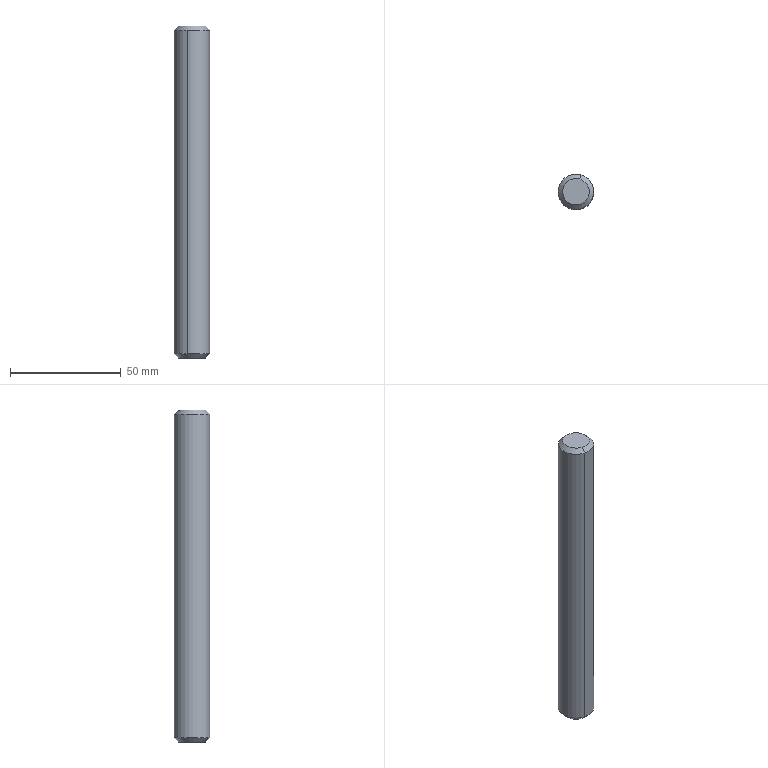Part | STEP file | Input 92 | 1 solid | 8 faces | box 16 x 16 x 150 mm | volume 29975 mm3 | cone 4 | cylinder 2 | plane 2 | commonest cylinder face diameters 16 x2
STEP:
#1=CARTESIAN_POINT('',(0.,0.,0.));
#2=DIRECTION('',(0.,0.,1.));
#3=DIRECTION('',(1.,0.,0.));
#4=AXIS2_PLACEMENT_3D('',#1,#2,#3);
#5=CARTESIAN_POINT('',(3968.69,438.757,-218.752));
#6=VERTEX_POINT('',#5);
#7=CARTESIAN_POINT('',(3965.31,427.243,-218.752));
#8=VERTEX_POINT('',#7);
#9=CARTESIAN_POINT('',(3967.,433.,-218.752));
#10=DIRECTION('',(0.,0.,1.));
#11=DIRECTION('',(0.2817,0.9595,0.));
#12=AXIS2_PLACEMENT_3D('',#9,#10,#11);
#13=CIRCLE('',#12,6.);
#14=CARTESIAN_POINT('',(3967.,433.,-218.752));
#15=DIRECTION('',(0.,0.,-1.));
#16=DIRECTION('',(-0.2817,-0.9595,0.));
#17=AXIS2_PLACEMENT_3D('',#14,#15,#16);
#18=CONICAL_SURFACE('',#17,6.,0.7854);
#19=CARTESIAN_POINT('',(3.142,0.));
#20=DIRECTION('',(-1.,0.));
#21=VECTOR('',#20,1.);
#22=LINE('',#19,#21);
#23=(GEOMETRIC_REPRESENTATION_CONTEXT(2)PARAMETRIC_REPRESENTATION_CONTEXT()REPRESENTATION_CONTEXT('',''));
#24=DEFINITIONAL_REPRESENTATION('',(#22),#23);
#25=PCURVE('',#18,#24);
#26=CARTESIAN_POINT('',(3967.,433.,-218.752));
#27=DIRECTION('',(0.,0.,1.));
#28=DIRECTION('',(0.2817,0.9595,0.));
#29=AXIS2_PLACEMENT_3D('',#26,#27,#28);
#30=PLANE('',#29);
#31=CARTESIAN_POINT('',(0.,0.));
#32=DIRECTION('',(1.,0.));
#33=AXIS2_PLACEMENT_2D('',#31,#32);
#34=CIRCLE('',#33,6.);
#35=(GEOMETRIC_REPRESENTATION_CONTEXT(2)PARAMETRIC_REPRESENTATION_CONTEXT()REPRESENTATION_CONTEXT('',''));
#36=DEFINITIONAL_REPRESENTATION('',(#34),#35);
#37=PCURVE('',#30,#36);
#38=SURFACE_CURVE('',#13,(#25,#37),.PCURVE_S1.);
#39=EDGE_CURVE('',#6,#8,#38,.T.);
#40=ORIENTED_EDGE('',*,*,#39,.F.);
#41=CARTESIAN_POINT('',(3969.254,440.676,-220.752));
#42=VERTEX_POINT('',#41);
#43=CARTESIAN_POINT('',(3968.69,438.757,-218.752));
#44=DIRECTION('',(0.1992,0.6785,-0.7071));
#45=VECTOR('',#44,1.);
#46=LINE('',#43,#45);
#47=CARTESIAN_POINT('',(3.142,0.));
#48=DIRECTION('',(0.,1.));
#49=VECTOR('',#48,1.);
#50=LINE('',#47,#49);
#51=(GEOMETRIC_REPRESENTATION_CONTEXT(2)PARAMETRIC_REPRESENTATION_CONTEXT()REPRESENTATION_CONTEXT('',''));
#52=DEFINITIONAL_REPRESENTATION('',(#50),#51);
#53=PCURVE('',#18,#52);
#54=CARTESIAN_POINT('',(3967.,433.,-218.752));
#55=DIRECTION('',(0.,0.,-1.));
#56=DIRECTION('',(-0.2817,-0.9595,0.));
#57=AXIS2_PLACEMENT_3D('',#54,#55,#56);
#58=CONICAL_SURFACE('',#57,6.,0.7854);
#59=CARTESIAN_POINT('',(3.142,0.));
#60=DIRECTION('',(0.,1.));
#61=VECTOR('',#60,1.);
#62=LINE('',#59,#61);
#63=(GEOMETRIC_REPRESENTATION_CONTEXT(2)PARAMETRIC_REPRESENTATION_CONTEXT()REPRESENTATION_CONTEXT('',''));
#64=DEFINITIONAL_REPRESENTATION('',(#62),#63);
#65=PCURVE('',#58,#64);
#66=SURFACE_CURVE('',#46,(#53,#65),.PCURVE_S1.);
#67=EDGE_CURVE('',#6,#42,#66,.T.);
#68=ORIENTED_EDGE('',*,*,#67,.T.);
#69=CARTESIAN_POINT('',(3964.746,425.324,-220.752));
#70=VERTEX_POINT('',#69);
#71=CARTESIAN_POINT('',(3967.,433.,-220.752));
#72=DIRECTION('',(0.,0.,-1.));
#73=DIRECTION('',(0.2817,0.9595,0.));
#74=AXIS2_PLACEMENT_3D('',#71,#72,#73);
#75=CIRCLE('',#74,8.);
#76=CARTESIAN_POINT('',(-3.142,2.));
#77=DIRECTION('',(1.,0.));
#78=VECTOR('',#77,1.);
#79=LINE('',#76,#78);
#80=(GEOMETRIC_REPRESENTATION_CONTEXT(2)PARAMETRIC_REPRESENTATION_CONTEXT()REPRESENTATION_CONTEXT('',''));
#81=DEFINITIONAL_REPRESENTATION('',(#79),#80);
#82=PCURVE('',#18,#81);
#83=CARTESIAN_POINT('',(3967.,433.,-218.752));
#84=DIRECTION('',(0.,0.,-1.));
#85=DIRECTION('',(-0.2817,-0.9595,0.));
#86=AXIS2_PLACEMENT_3D('',#83,#84,#85);
#87=CYLINDRICAL_SURFACE('',#86,8.);
#88=CARTESIAN_POINT('',(-3.142,2.));
#89=DIRECTION('',(1.,0.));
#90=VECTOR('',#89,1.);
#91=LINE('',#88,#90);
#92=(GEOMETRIC_REPRESENTATION_CONTEXT(2)PARAMETRIC_REPRESENTATION_CONTEXT()REPRESENTATION_CONTEXT('',''));
#93=DEFINITIONAL_REPRESENTATION('',(#91),#92);
#94=PCURVE('',#87,#93);
#95=SURFACE_CURVE('',#75,(#82,#94),.PCURVE_S1.);
#96=EDGE_CURVE('',#70,#42,#95,.T.);
#97=ORIENTED_EDGE('',*,*,#96,.F.);
#98=CARTESIAN_POINT('',(3965.31,427.243,-218.752));
#99=DIRECTION('',(-0.1992,-0.6785,-0.7071));
#100=VECTOR('',#99,1.);
#101=LINE('',#98,#100);
#102=CARTESIAN_POINT('',(0.,0.));
#103=DIRECTION('',(0.,1.));
#104=VECTOR('',#103,1.);
#105=LINE('',#102,#104);
#106=(GEOMETRIC_REPRESENTATION_CONTEXT(2)PARAMETRIC_REPRESENTATION_CONTEXT()REPRESENTATION_CONTEXT('',''));
#107=DEFINITIONAL_REPRESENTATION('',(#105),#106);
#108=PCURVE('',#18,#107);
#109=CARTESIAN_POINT('',(6.283,0.));
#110=DIRECTION('',(0.,1.));
#111=VECTOR('',#110,1.);
#112=LINE('',#109,#111);
#113=(GEOMETRIC_REPRESENTATION_CONTEXT(2)PARAMETRIC_REPRESENTATION_CONTEXT()REPRESENTATION_CONTEXT('',''));
#114=DEFINITIONAL_REPRESENTATION('',(#112),#113);
#115=PCURVE('',#58,#114);
#116=SURFACE_CURVE('',#101,(#108,#115),.PCURVE_S1.);
#117=EDGE_CURVE('',#8,#70,#116,.T.);
#118=ORIENTED_EDGE('',*,*,#117,.F.);
#119=EDGE_LOOP('',(#40,#68,#97,#118));
#120=FACE_BOUND('',#119,.T.);
#121=ADVANCED_FACE('',(#120),#18,.T.);
#122=CARTESIAN_POINT('',(3965.31,427.243,-368.752));
#123=VERTEX_POINT('',#122);
#124=CARTESIAN_POINT('',(3968.69,438.757,-368.752));
#125=VERTEX_POINT('',#124);
#126=CARTESIAN_POINT('',(3967.,433.,-368.752));
#127=DIRECTION('',(0.,0.,-1.));
#128=DIRECTION('',(0.2817,0.9595,0.));
#129=AXIS2_PLACEMENT_3D('',#126,#127,#128);
#130=CIRCLE('',#129,6.);
#131=CARTESIAN_POINT('',(3967.,433.,-366.752));
#132=DIRECTION('',(0.,0.,1.));
#133=DIRECTION('',(0.2817,0.9595,0.));
#134=AXIS2_PLACEMENT_3D('',#131,#132,#133);
#135=CONICAL_SURFACE('',#134,8.,0.7854);
#136=CARTESIAN_POINT('',(6.283,-2.));
#137=DIRECTION('',(-1.,0.));
#138=VECTOR('',#137,1.);
#139=LINE('',#136,#138);
#140=(GEOMETRIC_REPRESENTATION_CONTEXT(2)PARAMETRIC_REPRESENTATION_CONTEXT()REPRESENTATION_CONTEXT('',''));
#141=DEFINITIONAL_REPRESENTATION('',(#139),#140);
#142=PCURVE('',#135,#141);
#143=CARTESIAN_POINT('',(3967.,433.,-368.752));
#144=DIRECTION('',(0.,0.,1.));
#145=DIRECTION('',(0.2817,0.9595,0.));
#146=AXIS2_PLACEMENT_3D('',#143,#144,#145);
#147=PLANE('',#146);
#148=CARTESIAN_POINT('',(6.,0.));
#149=CARTESIAN_POINT('',(6.,-10.392));
#150=CARTESIAN_POINT('',(-3.,-5.196));
#151=CARTESIAN_POINT('',(-12.,0.));
#152=CARTESIAN_POINT('',(-3.,5.196));
#153=CARTESIAN_POINT('',(6.,10.392));
#154=CARTESIAN_POINT('',(6.,0.));
#155=(BOUNDED_CURVE()B_SPLINE_CURVE(2,(#148,#149,#150,#151,#152,#153,#154),.UNSPECIFIED.,.T.,.F.)B_SPLINE_CURVE_WITH_KNOTS((1,2,2,2,2,1),(-2.094,0.,2.094,4.189,6.283,8.378),.UNSPECIFIED.)CURVE()GEOMETRIC_REPRESENTATION_ITEM()RATIONAL_B_SPLINE_CURVE((1.,0.5,1.,0.5,1.,0.5,1.))REPRESENTATION_ITEM(''));
#156=(GEOMETRIC_REPRESENTATION_CONTEXT(2)PARAMETRIC_REPRESENTATION_CONTEXT()REPRESENTATION_CONTEXT('',''));
#157=DEFINITIONAL_REPRESENTATION('',(#155),#156);
#158=PCURVE('',#147,#157);
#159=SURFACE_CURVE('',#130,(#142,#158),.PCURVE_S1.);
#160=EDGE_CURVE('',#123,#125,#159,.T.);
#161=ORIENTED_EDGE('',*,*,#160,.F.);
#162=CARTESIAN_POINT('',(3964.746,425.324,-366.752));
#163=VERTEX_POINT('',#162);
#164=CARTESIAN_POINT('',(3964.746,425.324,-366.752));
#165=DIRECTION('',(-0.1992,-0.6785,0.7071));
#166=VECTOR('',#165,1.);
#167=LINE('',#164,#166);
#168=CARTESIAN_POINT('',(3.142,0.));
#169=DIRECTION('',(0.,1.));
#170=VECTOR('',#169,1.);
#171=LINE('',#168,#170);
#172=(GEOMETRIC_REPRESENTATION_CONTEXT(2)PARAMETRIC_REPRESENTATION_CONTEXT()REPRESENTATION_CONTEXT('',''));
#173=DEFINITIONAL_REPRESENTATION('',(#171),#172);
#174=PCURVE('',#135,#173);
#175=CARTESIAN_POINT('',(3967.,433.,-366.752));
#176=DIRECTION('',(0.,0.,1.));
#177=DIRECTION('',(0.2817,0.9595,0.));
#178=AXIS2_PLACEMENT_3D('',#175,#176,#177);
#179=CONICAL_SURFACE('',#178,8.,0.7854);
#180=CARTESIAN_POINT('',(3.142,0.));
#181=DIRECTION('',(0.,1.));
#182=VECTOR('',#181,1.);
#183=LINE('',#180,#182);
#184=(GEOMETRIC_REPRESENTATION_CONTEXT(2)PARAMETRIC_REPRESENTATION_CONTEXT()REPRESENTATION_CONTEXT('',''));
#185=DEFINITIONAL_REPRESENTATION('',(#183),#184);
#186=PCURVE('',#179,#185);
#187=SURFACE_CURVE('',#167,(#174,#186),.PCURVE_S1.);
#188=EDGE_CURVE('',#123,#163,#187,.T.);
#189=ORIENTED_EDGE('',*,*,#188,.T.);
#190=CARTESIAN_POINT('',(3969.254,440.676,-366.752));
#191=VERTEX_POINT('',#190);
#192=CARTESIAN_POINT('',(3967.,433.,-366.752));
#193=DIRECTION('',(0.,0.,1.));
#194=DIRECTION('',(0.2817,0.9595,0.));
#195=AXIS2_PLACEMENT_3D('',#192,#193,#194);
#196=CIRCLE('',#195,8.);
#197=CARTESIAN_POINT('',(0.,0.));
#198=DIRECTION('',(1.,0.));
#199=VECTOR('',#198,1.);
#200=LINE('',#197,#199);
#201=(GEOMETRIC_REPRESENTATION_CONTEXT(2)PARAMETRIC_REPRESENTATION_CONTEXT()REPRESENTATION_CONTEXT('',''));
#202=DEFINITIONAL_REPRESENTATION('',(#200),#201);
#203=PCURVE('',#135,#202);
#204=CARTESIAN_POINT('',(3.142,148.));
#205=DIRECTION('',(-1.,0.));
#206=VECTOR('',#205,1.);
#207=LINE('',#204,#206);
#208=(GEOMETRIC_REPRESENTATION_CONTEXT(2)PARAMETRIC_REPRESENTATION_CONTEXT()REPRESENTATION_CONTEXT('',''));
#209=DEFINITIONAL_REPRESENTATION('',(#207),#208);
#210=PCURVE('',#87,#209);
#211=SURFACE_CURVE('',#196,(#203,#210),.PCURVE_S1.);
#212=EDGE_CURVE('',#191,#163,#211,.T.);
#213=ORIENTED_EDGE('',*,*,#212,.F.);
#214=CARTESIAN_POINT('',(3969.254,440.676,-366.752));
#215=DIRECTION('',(0.1992,0.6785,0.7071));
#216=VECTOR('',#215,1.);
#217=LINE('',#214,#216);
#218=CARTESIAN_POINT('',(0.,0.));
#219=DIRECTION('',(0.,1.));
#220=VECTOR('',#219,1.);
#221=LINE('',#218,#220);
#222=(GEOMETRIC_REPRESENTATION_CONTEXT(2)PARAMETRIC_REPRESENTATION_CONTEXT()REPRESENTATION_CONTEXT('',''));
#223=DEFINITIONAL_REPRESENTATION('',(#221),#222);
#224=PCURVE('',#135,#223);
#225=CARTESIAN_POINT('',(6.283,0.));
#226=DIRECTION('',(0.,1.));
#227=VECTOR('',#226,1.);
#228=LINE('',#225,#227);
#229=(GEOMETRIC_REPRESENTATION_CONTEXT(2)PARAMETRIC_REPRESENTATION_CONTEXT()REPRESENTATION_CONTEXT('',''));
#230=DEFINITIONAL_REPRESENTATION('',(#228),#229);
#231=PCURVE('',#179,#230);
#232=SURFACE_CURVE('',#217,(#224,#231),.PCURVE_S1.);
#233=EDGE_CURVE('',#125,#191,#232,.T.);
#234=ORIENTED_EDGE('',*,*,#233,.F.);
#235=EDGE_LOOP('',(#161,#189,#213,#234));
#236=FACE_BOUND('',#235,.T.);
#237=ADVANCED_FACE('',(#236),#135,.T.);
#238=ORIENTED_EDGE('',*,*,#96,.T.);
#239=CARTESIAN_POINT('',(3969.254,440.676,-218.752));
#240=DIRECTION('',(0.,0.,-1.));
#241=VECTOR('',#240,1.);
#242=LINE('',#239,#241);
#243=CARTESIAN_POINT('',(3.142,0.));
#244=DIRECTION('',(0.,1.));
#245=VECTOR('',#244,1.);
#246=LINE('',#243,#245);
#247=(GEOMETRIC_REPRESENTATION_CONTEXT(2)PARAMETRIC_REPRESENTATION_CONTEXT()REPRESENTATION_CONTEXT('',''));
#248=DEFINITIONAL_REPRESENTATION('',(#246),#247);
#249=PCURVE('',#87,#248);
#250=CARTESIAN_POINT('',(3967.,433.,-218.752));
#251=DIRECTION('',(0.,0.,-1.));
#252=DIRECTION('',(-0.2817,-0.9595,0.));
#253=AXIS2_PLACEMENT_3D('',#250,#251,#252);
#254=CYLINDRICAL_SURFACE('',#253,8.);
#255=CARTESIAN_POINT('',(3.142,0.));
#256=DIRECTION('',(0.,1.));
#257=VECTOR('',#256,1.);
#258=LINE('',#255,#257);
#259=(GEOMETRIC_REPRESENTATION_CONTEXT(2)PARAMETRIC_REPRESENTATION_CONTEXT()REPRESENTATION_CONTEXT('',''));
#260=DEFINITIONAL_REPRESENTATION('',(#258),#259);
#261=PCURVE('',#254,#260);
#262=SURFACE_CURVE('',#242,(#249,#261),.PCURVE_S1.);
#263=EDGE_CURVE('',#42,#191,#262,.T.);
#264=ORIENTED_EDGE('',*,*,#263,.T.);
#265=ORIENTED_EDGE('',*,*,#212,.T.);
#266=CARTESIAN_POINT('',(3964.746,425.324,-218.752));
#267=DIRECTION('',(0.,0.,-1.));
#268=VECTOR('',#267,1.);
#269=LINE('',#266,#268);
#270=CARTESIAN_POINT('',(0.,0.));
#271=DIRECTION('',(0.,1.));
#272=VECTOR('',#271,1.);
#273=LINE('',#270,#272);
#274=(GEOMETRIC_REPRESENTATION_CONTEXT(2)PARAMETRIC_REPRESENTATION_CONTEXT()REPRESENTATION_CONTEXT('',''));
#275=DEFINITIONAL_REPRESENTATION('',(#273),#274);
#276=PCURVE('',#87,#275);
#277=CARTESIAN_POINT('',(6.283,0.));
#278=DIRECTION('',(0.,1.));
#279=VECTOR('',#278,1.);
#280=LINE('',#277,#279);
#281=(GEOMETRIC_REPRESENTATION_CONTEXT(2)PARAMETRIC_REPRESENTATION_CONTEXT()REPRESENTATION_CONTEXT('',''));
#282=DEFINITIONAL_REPRESENTATION('',(#280),#281);
#283=PCURVE('',#254,#282);
#284=SURFACE_CURVE('',#269,(#276,#283),.PCURVE_S1.);
#285=EDGE_CURVE('',#70,#163,#284,.T.);
#286=ORIENTED_EDGE('',*,*,#285,.F.);
#287=EDGE_LOOP('',(#238,#264,#265,#286));
#288=FACE_BOUND('',#287,.T.);
#289=ADVANCED_FACE('',(#288),#87,.T.);
#290=ORIENTED_EDGE('',*,*,#263,.F.);
#291=CARTESIAN_POINT('',(3967.,433.,-220.752));
#292=DIRECTION('',(0.,0.,-1.));
#293=DIRECTION('',(0.2817,0.9595,0.));
#294=AXIS2_PLACEMENT_3D('',#291,#292,#293);
#295=CIRCLE('',#294,8.);
#296=CARTESIAN_POINT('',(3.142,2.));
#297=DIRECTION('',(1.,0.));
#298=VECTOR('',#297,1.);
#299=LINE('',#296,#298);
#300=(GEOMETRIC_REPRESENTATION_CONTEXT(2)PARAMETRIC_REPRESENTATION_CONTEXT()REPRESENTATION_CONTEXT('',''));
#301=DEFINITIONAL_REPRESENTATION('',(#299),#300);
#302=PCURVE('',#254,#301);
#303=CARTESIAN_POINT('',(3.142,2.));
#304=DIRECTION('',(1.,0.));
#305=VECTOR('',#304,1.);
#306=LINE('',#303,#305);
#307=(GEOMETRIC_REPRESENTATION_CONTEXT(2)PARAMETRIC_REPRESENTATION_CONTEXT()REPRESENTATION_CONTEXT('',''));
#308=DEFINITIONAL_REPRESENTATION('',(#306),#307);
#309=PCURVE('',#58,#308);
#310=SURFACE_CURVE('',#295,(#302,#309),.PCURVE_S1.);
#311=EDGE_CURVE('',#42,#70,#310,.T.);
#312=ORIENTED_EDGE('',*,*,#311,.T.);
#313=ORIENTED_EDGE('',*,*,#285,.T.);
#314=CARTESIAN_POINT('',(3967.,433.,-366.752));
#315=DIRECTION('',(0.,0.,1.));
#316=DIRECTION('',(0.2817,0.9595,0.));
#317=AXIS2_PLACEMENT_3D('',#314,#315,#316);
#318=CIRCLE('',#317,8.);
#319=CARTESIAN_POINT('',(9.425,148.));
#320=DIRECTION('',(-1.,0.));
#321=VECTOR('',#320,1.);
#322=LINE('',#319,#321);
#323=(GEOMETRIC_REPRESENTATION_CONTEXT(2)PARAMETRIC_REPRESENTATION_CONTEXT()REPRESENTATION_CONTEXT('',''));
#324=DEFINITIONAL_REPRESENTATION('',(#322),#323);
#325=PCURVE('',#254,#324);
#326=CARTESIAN_POINT('',(0.,0.));
#327=DIRECTION('',(1.,0.));
#328=VECTOR('',#327,1.);
#329=LINE('',#326,#328);
#330=(GEOMETRIC_REPRESENTATION_CONTEXT(2)PARAMETRIC_REPRESENTATION_CONTEXT()REPRESENTATION_CONTEXT('',''));
#331=DEFINITIONAL_REPRESENTATION('',(#329),#330);
#332=PCURVE('',#179,#331);
#333=SURFACE_CURVE('',#318,(#325,#332),.PCURVE_S1.);
#334=EDGE_CURVE('',#163,#191,#333,.T.);
#335=ORIENTED_EDGE('',*,*,#334,.T.);
#336=EDGE_LOOP('',(#290,#312,#313,#335));
#337=FACE_BOUND('',#336,.T.);
#338=ADVANCED_FACE('',(#337),#254,.T.);
#339=CARTESIAN_POINT('',(3967.,433.,-218.752));
#340=DIRECTION('',(0.,0.,1.));
#341=DIRECTION('',(0.2817,0.9595,0.));
#342=AXIS2_PLACEMENT_3D('',#339,#340,#341);
#343=CIRCLE('',#342,6.);
#344=CARTESIAN_POINT('',(0.,0.));
#345=DIRECTION('',(1.,0.));
#346=AXIS2_PLACEMENT_2D('',#344,#345);
#347=CIRCLE('',#346,6.);
#348=(GEOMETRIC_REPRESENTATION_CONTEXT(2)PARAMETRIC_REPRESENTATION_CONTEXT()REPRESENTATION_CONTEXT('',''));
#349=DEFINITIONAL_REPRESENTATION('',(#347),#348);
#350=PCURVE('',#30,#349);
#351=CARTESIAN_POINT('',(9.425,0.));
#352=DIRECTION('',(-1.,0.));
#353=VECTOR('',#352,1.);
#354=LINE('',#351,#353);
#355=(GEOMETRIC_REPRESENTATION_CONTEXT(2)PARAMETRIC_REPRESENTATION_CONTEXT()REPRESENTATION_CONTEXT('',''));
#356=DEFINITIONAL_REPRESENTATION('',(#354),#355);
#357=PCURVE('',#58,#356);
#358=SURFACE_CURVE('',#343,(#350,#357),.PCURVE_S1.);
#359=EDGE_CURVE('',#8,#6,#358,.T.);
#360=ORIENTED_EDGE('',*,*,#359,.T.);
#361=ORIENTED_EDGE('',*,*,#39,.T.);
#362=EDGE_LOOP('',(#360,#361));
#363=FACE_BOUND('',#362,.T.);
#364=ADVANCED_FACE('',(#363),#30,.T.);
#365=CARTESIAN_POINT('',(3967.,433.,-368.752));
#366=DIRECTION('',(0.,0.,-1.));
#367=DIRECTION('',(0.2817,0.9595,0.));
#368=AXIS2_PLACEMENT_3D('',#365,#366,#367);
#369=CIRCLE('',#368,6.);
#370=CARTESIAN_POINT('',(6.,0.));
#371=CARTESIAN_POINT('',(6.,-10.392));
#372=CARTESIAN_POINT('',(-3.,-5.196));
#373=CARTESIAN_POINT('',(-12.,0.));
#374=CARTESIAN_POINT('',(-3.,5.196));
#375=CARTESIAN_POINT('',(6.,10.392));
#376=CARTESIAN_POINT('',(6.,0.));
#377=(BOUNDED_CURVE()B_SPLINE_CURVE(2,(#370,#371,#372,#373,#374,#375,#376),.UNSPECIFIED.,.T.,.F.)B_SPLINE_CURVE_WITH_KNOTS((1,2,2,2,2,1),(-2.094,0.,2.094,4.189,6.283,8.378),.UNSPECIFIED.)CURVE()GEOMETRIC_REPRESENTATION_ITEM()RATIONAL_B_SPLINE_CURVE((1.,0.5,1.,0.5,1.,0.5,1.))REPRESENTATION_ITEM(''));
#378=(GEOMETRIC_REPRESENTATION_CONTEXT(2)PARAMETRIC_REPRESENTATION_CONTEXT()REPRESENTATION_CONTEXT('',''));
#379=DEFINITIONAL_REPRESENTATION('',(#377),#378);
#380=PCURVE('',#147,#379);
#381=CARTESIAN_POINT('',(6.283,-2.));
#382=DIRECTION('',(-1.,0.));
#383=VECTOR('',#382,1.);
#384=LINE('',#381,#383);
#385=(GEOMETRIC_REPRESENTATION_CONTEXT(2)PARAMETRIC_REPRESENTATION_CONTEXT()REPRESENTATION_CONTEXT('',''));
#386=DEFINITIONAL_REPRESENTATION('',(#384),#385);
#387=PCURVE('',#179,#386);
#388=SURFACE_CURVE('',#369,(#380,#387),.PCURVE_S1.);
#389=EDGE_CURVE('',#125,#123,#388,.T.);
#390=ORIENTED_EDGE('',*,*,#389,.T.);
#391=ORIENTED_EDGE('',*,*,#160,.T.);
#392=EDGE_LOOP('',(#390,#391));
#393=FACE_BOUND('',#392,.T.);
#394=ADVANCED_FACE('',(#393),#147,.F.);
#395=ORIENTED_EDGE('',*,*,#188,.F.);
#396=ORIENTED_EDGE('',*,*,#389,.F.);
#397=ORIENTED_EDGE('',*,*,#233,.T.);
#398=ORIENTED_EDGE('',*,*,#334,.F.);
#399=EDGE_LOOP('',(#395,#396,#397,#398));
#400=FACE_BOUND('',#399,.T.);
#401=ADVANCED_FACE('',(#400),#179,.T.);
#402=ORIENTED_EDGE('',*,*,#67,.F.);
#403=ORIENTED_EDGE('',*,*,#359,.F.);
#404=ORIENTED_EDGE('',*,*,#117,.T.);
#405=ORIENTED_EDGE('',*,*,#311,.F.);
#406=EDGE_LOOP('',(#402,#403,#404,#405));
#407=FACE_BOUND('',#406,.T.);
#408=ADVANCED_FACE('',(#407),#58,.T.);
#409=CLOSED_SHELL('',(#121,#237,#289,#338,#364,#394,#401,#408));
#410=MANIFOLD_SOLID_BREP('',#409);
#411=(LENGTH_UNIT()NAMED_UNIT(*)SI_UNIT(.MILLI.,.METRE.));
#412=UNCERTAINTY_MEASURE_WITH_UNIT(LENGTH_MEASURE(0.0000001),#411,'','');
#413=(NAMED_UNIT(*)PLANE_ANGLE_UNIT()SI_UNIT($,.RADIAN.));
#414=(NAMED_UNIT(*)SI_UNIT($,.STERADIAN.)SOLID_ANGLE_UNIT());
#415=(GEOMETRIC_REPRESENTATION_CONTEXT(3)GLOBAL_UNCERTAINTY_ASSIGNED_CONTEXT((#412))GLOBAL_UNIT_ASSIGNED_CONTEXT((#411,#413,#414))REPRESENTATION_CONTEXT('',''));
#416=ADVANCED_BREP_SHAPE_REPRESENTATION('',(#4,#410),#415);